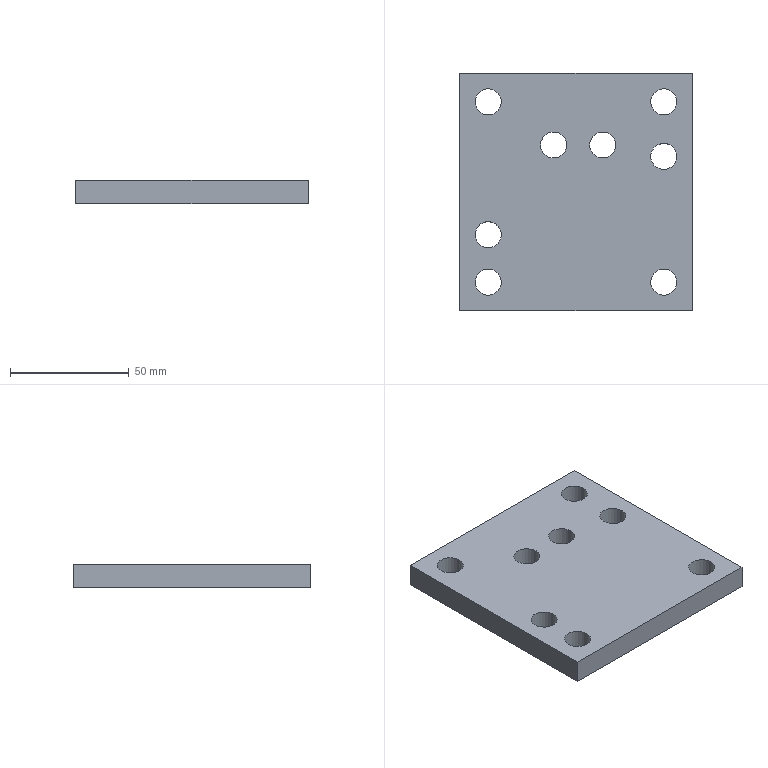Part | NX | features solid 2 | 1 solid | 14 faces | box 98 x 100 x 10 mm | volume 90397 mm3 | cylinder 8 | plane 6 | commonest cylinder face diameters 11 x8
STEP:
#1=CARTESIAN_POINT('',(495.719,-63.299,88.));
#2=VERTEX_POINT('',#1);
#3=CARTESIAN_POINT('',(495.719,-63.299,78.));
#4=VERTEX_POINT('',#3);
#5=CARTESIAN_POINT('',(495.719,-63.299,78.));
#6=DIRECTION('',(0.,0.,1.));
#7=VECTOR('',#6,1000.);
#8=LINE('',#5,#7);
#9=EDGE_CURVE('',#2,#4,#8,.F.);
#10=ORIENTED_EDGE('',*,*,#9,.F.);
#11=CARTESIAN_POINT('',(397.719,-63.299,88.));
#12=VERTEX_POINT('',#11);
#13=CARTESIAN_POINT('',(287.,-63.299,88.));
#14=DIRECTION('',(-1.,0.,0.));
#15=VECTOR('',#14,1000.);
#16=LINE('',#13,#15);
#17=EDGE_CURVE('',#12,#2,#16,.F.);
#18=ORIENTED_EDGE('',*,*,#17,.F.);
#19=CARTESIAN_POINT('',(397.719,-63.299,78.));
#20=VERTEX_POINT('',#19);
#21=CARTESIAN_POINT('',(397.719,-63.299,78.));
#22=DIRECTION('',(0.,0.,1.));
#23=VECTOR('',#22,1000.);
#24=LINE('',#21,#23);
#25=EDGE_CURVE('',#12,#20,#24,.F.);
#26=ORIENTED_EDGE('',*,*,#25,.T.);
#27=CARTESIAN_POINT('',(446.479,-63.299,78.));
#28=DIRECTION('',(-1.,0.,0.));
#29=VECTOR('',#28,1000.);
#30=LINE('',#27,#29);
#31=EDGE_CURVE('',#20,#4,#30,.F.);
#32=ORIENTED_EDGE('',*,*,#31,.T.);
#33=EDGE_LOOP('',(#10,#18,#26,#32));
#34=FACE_BOUND('',#33,.T.);
#35=CARTESIAN_POINT('',(446.479,-63.299,78.));
#36=DIRECTION('',(0.,1.,0.));
#37=DIRECTION('',(-1.,0.,0.));
#38=AXIS2_PLACEMENT_3D('',#35,#36,#37);
#39=PLANE('',#38);
#40=ADVANCED_FACE('',(#34),#39,.F.);
#41=ORIENTED_EDGE('',*,*,#25,.F.);
#42=CARTESIAN_POINT('',(397.719,36.701,88.));
#43=VERTEX_POINT('',#42);
#44=CARTESIAN_POINT('',(397.719,-0.000000688,88.));
#45=DIRECTION('',(0.,-1.,0.));
#46=VECTOR('',#45,1000.);
#47=LINE('',#44,#46);
#48=EDGE_CURVE('',#43,#12,#47,.T.);
#49=ORIENTED_EDGE('',*,*,#48,.F.);
#50=CARTESIAN_POINT('',(397.719,36.701,78.));
#51=VERTEX_POINT('',#50);
#52=CARTESIAN_POINT('',(397.719,36.701,78.));
#53=DIRECTION('',(0.,0.,1.));
#54=VECTOR('',#53,1000.);
#55=LINE('',#52,#54);
#56=EDGE_CURVE('',#43,#51,#55,.F.);
#57=ORIENTED_EDGE('',*,*,#56,.T.);
#58=CARTESIAN_POINT('',(397.719,-13.399,78.));
#59=DIRECTION('',(0.,1.,0.));
#60=VECTOR('',#59,1000.);
#61=LINE('',#58,#60);
#62=EDGE_CURVE('',#51,#20,#61,.F.);
#63=ORIENTED_EDGE('',*,*,#62,.T.);
#64=EDGE_LOOP('',(#41,#49,#57,#63));
#65=FACE_BOUND('',#64,.T.);
#66=CARTESIAN_POINT('',(397.719,-13.399,78.));
#67=DIRECTION('',(1.,0.,0.));
#68=DIRECTION('',(0.,1.,0.));
#69=AXIS2_PLACEMENT_3D('',#66,#67,#68);
#70=PLANE('',#69);
#71=ADVANCED_FACE('',(#65),#70,.F.);
#72=ORIENTED_EDGE('',*,*,#56,.F.);
#73=CARTESIAN_POINT('',(495.719,36.701,88.));
#74=VERTEX_POINT('',#73);
#75=CARTESIAN_POINT('',(287.,36.701,88.));
#76=DIRECTION('',(-1.,0.,0.));
#77=VECTOR('',#76,1000.);
#78=LINE('',#75,#77);
#79=EDGE_CURVE('',#74,#43,#78,.T.);
#80=ORIENTED_EDGE('',*,*,#79,.F.);
#81=CARTESIAN_POINT('',(495.719,36.701,78.));
#82=VERTEX_POINT('',#81);
#83=CARTESIAN_POINT('',(495.719,36.701,78.));
#84=DIRECTION('',(0.,0.,1.));
#85=VECTOR('',#84,1000.);
#86=LINE('',#83,#85);
#87=EDGE_CURVE('',#74,#82,#86,.F.);
#88=ORIENTED_EDGE('',*,*,#87,.T.);
#89=CARTESIAN_POINT('',(446.479,36.701,78.));
#90=DIRECTION('',(1.,0.,0.));
#91=VECTOR('',#90,1000.);
#92=LINE('',#89,#91);
#93=EDGE_CURVE('',#82,#51,#92,.F.);
#94=ORIENTED_EDGE('',*,*,#93,.T.);
#95=EDGE_LOOP('',(#72,#80,#88,#94));
#96=FACE_BOUND('',#95,.T.);
#97=CARTESIAN_POINT('',(446.479,36.701,78.));
#98=DIRECTION('',(0.,-1.,0.));
#99=DIRECTION('',(1.,0.,0.));
#100=AXIS2_PLACEMENT_3D('',#97,#98,#99);
#101=PLANE('',#100);
#102=ADVANCED_FACE('',(#96),#101,.F.);
#103=CARTESIAN_POINT('',(478.219,1.701,78.));
#104=VERTEX_POINT('',#103);
#105=CARTESIAN_POINT('',(483.719,1.701,78.));
#106=DIRECTION('',(0.,0.,1.));
#107=DIRECTION('',(-1.,0.,0.));
#108=AXIS2_PLACEMENT_3D('',#105,#106,#107);
#109=CIRCLE('',#108,5.5);
#110=EDGE_CURVE('',#104,#104,#109,.F.);
#111=ORIENTED_EDGE('',*,*,#110,.T.);
#112=EDGE_LOOP('',(#111));
#113=FACE_BOUND('',#112,.T.);
#114=CARTESIAN_POINT('',(478.219,1.701,88.));
#115=VERTEX_POINT('',#114);
#116=CARTESIAN_POINT('',(483.719,1.701,88.));
#117=DIRECTION('',(0.,0.,1.));
#118=DIRECTION('',(-1.,0.,0.));
#119=AXIS2_PLACEMENT_3D('',#116,#117,#118);
#120=CIRCLE('',#119,5.5);
#121=EDGE_CURVE('',#115,#115,#120,.F.);
#122=ORIENTED_EDGE('',*,*,#121,.F.);
#123=EDGE_LOOP('',(#122));
#124=FACE_BOUND('',#123,.T.);
#125=CARTESIAN_POINT('',(483.719,1.701,78.));
#126=DIRECTION('',(0.,0.,-1.));
#127=DIRECTION('',(-1.,0.,0.));
#128=AXIS2_PLACEMENT_3D('',#125,#126,#127);
#129=CYLINDRICAL_SURFACE('',#128,5.5);
#130=ADVANCED_FACE('',(#113,#124),#129,.F.);
#131=CARTESIAN_POINT('',(404.219,-31.299,78.));
#132=VERTEX_POINT('',#131);
#133=CARTESIAN_POINT('',(409.719,-31.299,78.));
#134=DIRECTION('',(0.,0.,1.));
#135=DIRECTION('',(-1.,0.,0.));
#136=AXIS2_PLACEMENT_3D('',#133,#134,#135);
#137=CIRCLE('',#136,5.5);
#138=EDGE_CURVE('',#132,#132,#137,.F.);
#139=ORIENTED_EDGE('',*,*,#138,.T.);
#140=EDGE_LOOP('',(#139));
#141=FACE_BOUND('',#140,.T.);
#142=CARTESIAN_POINT('',(404.219,-31.299,88.));
#143=VERTEX_POINT('',#142);
#144=CARTESIAN_POINT('',(409.719,-31.299,88.));
#145=DIRECTION('',(0.,0.,1.));
#146=DIRECTION('',(-1.,0.,0.));
#147=AXIS2_PLACEMENT_3D('',#144,#145,#146);
#148=CIRCLE('',#147,5.5);
#149=EDGE_CURVE('',#143,#143,#148,.F.);
#150=ORIENTED_EDGE('',*,*,#149,.F.);
#151=EDGE_LOOP('',(#150));
#152=FACE_BOUND('',#151,.T.);
#153=CARTESIAN_POINT('',(409.719,-31.299,78.));
#154=DIRECTION('',(0.,0.,-1.));
#155=DIRECTION('',(-1.,0.,0.));
#156=AXIS2_PLACEMENT_3D('',#153,#154,#155);
#157=CYLINDRICAL_SURFACE('',#156,5.5);
#158=ADVANCED_FACE('',(#141,#152),#157,.F.);
#159=CARTESIAN_POINT('',(404.219,-51.299,78.));
#160=VERTEX_POINT('',#159);
#161=CARTESIAN_POINT('',(409.719,-51.299,78.));
#162=DIRECTION('',(0.,0.,1.));
#163=DIRECTION('',(-1.,0.,0.));
#164=AXIS2_PLACEMENT_3D('',#161,#162,#163);
#165=CIRCLE('',#164,5.5);
#166=EDGE_CURVE('',#160,#160,#165,.T.);
#167=ORIENTED_EDGE('',*,*,#166,.F.);
#168=EDGE_LOOP('',(#167));
#169=FACE_BOUND('',#168,.T.);
#170=CARTESIAN_POINT('',(404.219,-51.299,88.));
#171=VERTEX_POINT('',#170);
#172=CARTESIAN_POINT('',(409.719,-51.299,88.));
#173=DIRECTION('',(0.,0.,1.));
#174=DIRECTION('',(-1.,0.,0.));
#175=AXIS2_PLACEMENT_3D('',#172,#173,#174);
#176=CIRCLE('',#175,5.5);
#177=EDGE_CURVE('',#171,#171,#176,.T.);
#178=ORIENTED_EDGE('',*,*,#177,.T.);
#179=EDGE_LOOP('',(#178));
#180=FACE_BOUND('',#179,.T.);
#181=CARTESIAN_POINT('',(409.719,-51.299,78.));
#182=DIRECTION('',(0.,0.,-1.));
#183=DIRECTION('',(-1.,0.,0.));
#184=AXIS2_PLACEMENT_3D('',#181,#182,#183);
#185=CYLINDRICAL_SURFACE('',#184,5.5);
#186=ADVANCED_FACE('',(#169,#180),#185,.F.);
#187=CARTESIAN_POINT('',(478.219,-51.299,78.));
#188=VERTEX_POINT('',#187);
#189=CARTESIAN_POINT('',(483.719,-51.299,78.));
#190=DIRECTION('',(0.,0.,1.));
#191=DIRECTION('',(-1.,0.,0.));
#192=AXIS2_PLACEMENT_3D('',#189,#190,#191);
#193=CIRCLE('',#192,5.5);
#194=EDGE_CURVE('',#188,#188,#193,.T.);
#195=ORIENTED_EDGE('',*,*,#194,.F.);
#196=EDGE_LOOP('',(#195));
#197=FACE_BOUND('',#196,.T.);
#198=CARTESIAN_POINT('',(478.219,-51.299,88.));
#199=VERTEX_POINT('',#198);
#200=CARTESIAN_POINT('',(483.719,-51.299,88.));
#201=DIRECTION('',(0.,0.,1.));
#202=DIRECTION('',(-1.,0.,0.));
#203=AXIS2_PLACEMENT_3D('',#200,#201,#202);
#204=CIRCLE('',#203,5.5);
#205=EDGE_CURVE('',#199,#199,#204,.T.);
#206=ORIENTED_EDGE('',*,*,#205,.T.);
#207=EDGE_LOOP('',(#206));
#208=FACE_BOUND('',#207,.T.);
#209=CARTESIAN_POINT('',(483.719,-51.299,78.));
#210=DIRECTION('',(0.,0.,-1.));
#211=DIRECTION('',(-1.,0.,0.));
#212=AXIS2_PLACEMENT_3D('',#209,#210,#211);
#213=CYLINDRICAL_SURFACE('',#212,5.5);
#214=ADVANCED_FACE('',(#197,#208),#213,.F.);
#215=CARTESIAN_POINT('',(478.219,24.701,78.));
#216=VERTEX_POINT('',#215);
#217=CARTESIAN_POINT('',(483.719,24.701,78.));
#218=DIRECTION('',(0.,0.,1.));
#219=DIRECTION('',(-1.,0.,0.));
#220=AXIS2_PLACEMENT_3D('',#217,#218,#219);
#221=CIRCLE('',#220,5.5);
#222=EDGE_CURVE('',#216,#216,#221,.T.);
#223=ORIENTED_EDGE('',*,*,#222,.F.);
#224=EDGE_LOOP('',(#223));
#225=FACE_BOUND('',#224,.T.);
#226=CARTESIAN_POINT('',(478.219,24.701,88.));
#227=VERTEX_POINT('',#226);
#228=CARTESIAN_POINT('',(483.719,24.701,88.));
#229=DIRECTION('',(0.,0.,1.));
#230=DIRECTION('',(-1.,0.,0.));
#231=AXIS2_PLACEMENT_3D('',#228,#229,#230);
#232=CIRCLE('',#231,5.5);
#233=EDGE_CURVE('',#227,#227,#232,.T.);
#234=ORIENTED_EDGE('',*,*,#233,.T.);
#235=EDGE_LOOP('',(#234));
#236=FACE_BOUND('',#235,.T.);
#237=CARTESIAN_POINT('',(483.719,24.701,78.));
#238=DIRECTION('',(0.,0.,-1.));
#239=DIRECTION('',(-1.,0.,0.));
#240=AXIS2_PLACEMENT_3D('',#237,#238,#239);
#241=CYLINDRICAL_SURFACE('',#240,5.5);
#242=ADVANCED_FACE('',(#225,#236),#241,.F.);
#243=CARTESIAN_POINT('',(404.219,24.701,78.));
#244=VERTEX_POINT('',#243);
#245=CARTESIAN_POINT('',(409.719,24.701,78.));
#246=DIRECTION('',(0.,0.,1.));
#247=DIRECTION('',(-1.,0.,0.));
#248=AXIS2_PLACEMENT_3D('',#245,#246,#247);
#249=CIRCLE('',#248,5.5);
#250=EDGE_CURVE('',#244,#244,#249,.F.);
#251=ORIENTED_EDGE('',*,*,#250,.T.);
#252=EDGE_LOOP('',(#251));
#253=FACE_BOUND('',#252,.T.);
#254=CARTESIAN_POINT('',(404.219,24.701,88.));
#255=VERTEX_POINT('',#254);
#256=CARTESIAN_POINT('',(409.719,24.701,88.));
#257=DIRECTION('',(0.,0.,1.));
#258=DIRECTION('',(-1.,0.,0.));
#259=AXIS2_PLACEMENT_3D('',#256,#257,#258);
#260=CIRCLE('',#259,5.5);
#261=EDGE_CURVE('',#255,#255,#260,.F.);
#262=ORIENTED_EDGE('',*,*,#261,.F.);
#263=EDGE_LOOP('',(#262));
#264=FACE_BOUND('',#263,.T.);
#265=CARTESIAN_POINT('',(409.719,24.701,78.));
#266=DIRECTION('',(0.,0.,-1.));
#267=DIRECTION('',(-1.,0.,0.));
#268=AXIS2_PLACEMENT_3D('',#265,#266,#267);
#269=CYLINDRICAL_SURFACE('',#268,5.5);
#270=ADVANCED_FACE('',(#253,#264),#269,.F.);
#271=CARTESIAN_POINT('',(495.719,-0.000000688,88.));
#272=DIRECTION('',(0.,-1.,0.));
#273=VECTOR('',#272,1000.);
#274=LINE('',#271,#273);
#275=EDGE_CURVE('',#2,#74,#274,.F.);
#276=ORIENTED_EDGE('',*,*,#275,.F.);
#277=ORIENTED_EDGE('',*,*,#9,.T.);
#278=CARTESIAN_POINT('',(495.719,-13.399,78.));
#279=DIRECTION('',(0.,-1.,0.));
#280=VECTOR('',#279,1000.);
#281=LINE('',#278,#280);
#282=EDGE_CURVE('',#4,#82,#281,.F.);
#283=ORIENTED_EDGE('',*,*,#282,.T.);
#284=ORIENTED_EDGE('',*,*,#87,.F.);
#285=EDGE_LOOP('',(#276,#277,#283,#284));
#286=FACE_BOUND('',#285,.T.);
#287=CARTESIAN_POINT('',(495.719,-13.399,78.));
#288=DIRECTION('',(-1.,0.,0.));
#289=DIRECTION('',(0.,-1.,0.));
#290=AXIS2_PLACEMENT_3D('',#287,#288,#289);
#291=PLANE('',#290);
#292=ADVANCED_FACE('',(#286),#291,.F.);
#293=CARTESIAN_POINT('',(452.471,6.5,78.));
#294=VERTEX_POINT('',#293);
#295=CARTESIAN_POINT('',(457.971,6.5,78.));
#296=DIRECTION('',(0.000000369,-0.000000231,1.));
#297=DIRECTION('',(-1.,0.,0.000000369));
#298=AXIS2_PLACEMENT_3D('',#295,#296,#297);
#299=CIRCLE('',#298,5.5);
#300=EDGE_CURVE('',#294,#294,#299,.T.);
#301=ORIENTED_EDGE('',*,*,#300,.F.);
#302=EDGE_LOOP('',(#301));
#303=FACE_BOUND('',#302,.T.);
#304=CARTESIAN_POINT('',(452.471,6.5,88.));
#305=VERTEX_POINT('',#304);
#306=CARTESIAN_POINT('',(457.971,6.5,88.));
#307=DIRECTION('',(0.000000369,-0.000000231,1.));
#308=DIRECTION('',(-1.,0.,0.000000369));
#309=AXIS2_PLACEMENT_3D('',#306,#307,#308);
#310=CIRCLE('',#309,5.5);
#311=EDGE_CURVE('',#305,#305,#310,.T.);
#312=ORIENTED_EDGE('',*,*,#311,.T.);
#313=EDGE_LOOP('',(#312));
#314=FACE_BOUND('',#313,.T.);
#315=CARTESIAN_POINT('',(457.971,6.5,78.));
#316=DIRECTION('',(-0.000000369,0.000000231,-1.));
#317=DIRECTION('',(-1.,0.,0.000000369));
#318=AXIS2_PLACEMENT_3D('',#315,#316,#317);
#319=CYLINDRICAL_SURFACE('',#318,5.5);
#320=ADVANCED_FACE('',(#303,#314),#319,.F.);
#321=CARTESIAN_POINT('',(431.763,6.5,78.));
#322=VERTEX_POINT('',#321);
#323=CARTESIAN_POINT('',(437.263,6.5,78.));
#324=DIRECTION('',(0.000000369,-0.000000231,1.));
#325=DIRECTION('',(-1.,0.,0.000000369));
#326=AXIS2_PLACEMENT_3D('',#323,#324,#325);
#327=CIRCLE('',#326,5.5);
#328=EDGE_CURVE('',#322,#322,#327,.F.);
#329=ORIENTED_EDGE('',*,*,#328,.T.);
#330=EDGE_LOOP('',(#329));
#331=FACE_BOUND('',#330,.T.);
#332=CARTESIAN_POINT('',(431.763,6.5,88.));
#333=VERTEX_POINT('',#332);
#334=CARTESIAN_POINT('',(437.263,6.5,88.));
#335=DIRECTION('',(0.000000369,-0.000000231,1.));
#336=DIRECTION('',(-1.,0.,0.000000369));
#337=AXIS2_PLACEMENT_3D('',#334,#335,#336);
#338=CIRCLE('',#337,5.5);
#339=EDGE_CURVE('',#333,#333,#338,.F.);
#340=ORIENTED_EDGE('',*,*,#339,.F.);
#341=EDGE_LOOP('',(#340));
#342=FACE_BOUND('',#341,.T.);
#343=CARTESIAN_POINT('',(437.263,6.5,78.));
#344=DIRECTION('',(-0.000000369,0.000000231,-1.));
#345=DIRECTION('',(-1.,0.,0.000000369));
#346=AXIS2_PLACEMENT_3D('',#343,#344,#345);
#347=CYLINDRICAL_SURFACE('',#346,5.5);
#348=ADVANCED_FACE('',(#331,#342),#347,.F.);
#349=ORIENTED_EDGE('',*,*,#300,.T.);
#350=EDGE_LOOP('',(#349));
#351=FACE_BOUND('',#350,.T.);
#352=ORIENTED_EDGE('',*,*,#328,.F.);
#353=EDGE_LOOP('',(#352));
#354=FACE_BOUND('',#353,.T.);
#355=ORIENTED_EDGE('',*,*,#110,.F.);
#356=EDGE_LOOP('',(#355));
#357=FACE_BOUND('',#356,.T.);
#358=ORIENTED_EDGE('',*,*,#138,.F.);
#359=EDGE_LOOP('',(#358));
#360=FACE_BOUND('',#359,.T.);
#361=ORIENTED_EDGE('',*,*,#166,.T.);
#362=EDGE_LOOP('',(#361));
#363=FACE_BOUND('',#362,.T.);
#364=ORIENTED_EDGE('',*,*,#194,.T.);
#365=EDGE_LOOP('',(#364));
#366=FACE_BOUND('',#365,.T.);
#367=ORIENTED_EDGE('',*,*,#222,.T.);
#368=EDGE_LOOP('',(#367));
#369=FACE_BOUND('',#368,.T.);
#370=ORIENTED_EDGE('',*,*,#250,.F.);
#371=EDGE_LOOP('',(#370));
#372=FACE_BOUND('',#371,.T.);
#373=ORIENTED_EDGE('',*,*,#93,.F.);
#374=ORIENTED_EDGE('',*,*,#282,.F.);
#375=ORIENTED_EDGE('',*,*,#31,.F.);
#376=ORIENTED_EDGE('',*,*,#62,.F.);
#377=EDGE_LOOP('',(#373,#374,#375,#376));
#378=FACE_BOUND('',#377,.T.);
#379=CARTESIAN_POINT('',(287.,-0.000000688,78.));
#380=DIRECTION('',(0.,0.,-1.));
#381=DIRECTION('',(-1.,0.,0.));
#382=AXIS2_PLACEMENT_3D('',#379,#380,#381);
#383=PLANE('',#382);
#384=ADVANCED_FACE('',(#351,#354,#357,#360,#363,#366,#369,#372,#378),#383,.T.);
#385=ORIENTED_EDGE('',*,*,#311,.F.);
#386=EDGE_LOOP('',(#385));
#387=FACE_BOUND('',#386,.T.);
#388=ORIENTED_EDGE('',*,*,#339,.T.);
#389=EDGE_LOOP('',(#388));
#390=FACE_BOUND('',#389,.T.);
#391=ORIENTED_EDGE('',*,*,#121,.T.);
#392=EDGE_LOOP('',(#391));
#393=FACE_BOUND('',#392,.T.);
#394=ORIENTED_EDGE('',*,*,#149,.T.);
#395=EDGE_LOOP('',(#394));
#396=FACE_BOUND('',#395,.T.);
#397=ORIENTED_EDGE('',*,*,#177,.F.);
#398=EDGE_LOOP('',(#397));
#399=FACE_BOUND('',#398,.T.);
#400=ORIENTED_EDGE('',*,*,#205,.F.);
#401=EDGE_LOOP('',(#400));
#402=FACE_BOUND('',#401,.T.);
#403=ORIENTED_EDGE('',*,*,#233,.F.);
#404=EDGE_LOOP('',(#403));
#405=FACE_BOUND('',#404,.T.);
#406=ORIENTED_EDGE('',*,*,#261,.T.);
#407=EDGE_LOOP('',(#406));
#408=FACE_BOUND('',#407,.T.);
#409=ORIENTED_EDGE('',*,*,#79,.T.);
#410=ORIENTED_EDGE('',*,*,#48,.T.);
#411=ORIENTED_EDGE('',*,*,#17,.T.);
#412=ORIENTED_EDGE('',*,*,#275,.T.);
#413=EDGE_LOOP('',(#409,#410,#411,#412));
#414=FACE_BOUND('',#413,.T.);
#415=CARTESIAN_POINT('',(287.,-0.000000688,88.));
#416=DIRECTION('',(0.,0.,-1.));
#417=DIRECTION('',(-1.,0.,0.));
#418=AXIS2_PLACEMENT_3D('',#415,#416,#417);
#419=PLANE('',#418);
#420=ADVANCED_FACE('',(#387,#390,#393,#396,#399,#402,#405,#408,#414),#419,.F.);
#421=CLOSED_SHELL('',(#40,#71,#102,#130,#158,#186,#214,#242,#270,#292,#320,#348,#384,#420));
#422=MANIFOLD_SOLID_BREP('',#421);
#423=(LENGTH_UNIT()NAMED_UNIT(*)SI_UNIT(.MILLI.,.METRE.));
#424=UNCERTAINTY_MEASURE_WITH_UNIT(LENGTH_MEASURE(0.00001),#423,'','');
#425=(NAMED_UNIT(*)PLANE_ANGLE_UNIT()SI_UNIT($,.RADIAN.));
#426=(NAMED_UNIT(*)SI_UNIT($,.STERADIAN.)SOLID_ANGLE_UNIT());
#427=(GEOMETRIC_REPRESENTATION_CONTEXT(3)GLOBAL_UNCERTAINTY_ASSIGNED_CONTEXT((#424))GLOBAL_UNIT_ASSIGNED_CONTEXT((#423,#425,#426))REPRESENTATION_CONTEXT('',''));
#428=ADVANCED_BREP_SHAPE_REPRESENTATION('',(#422),#427);